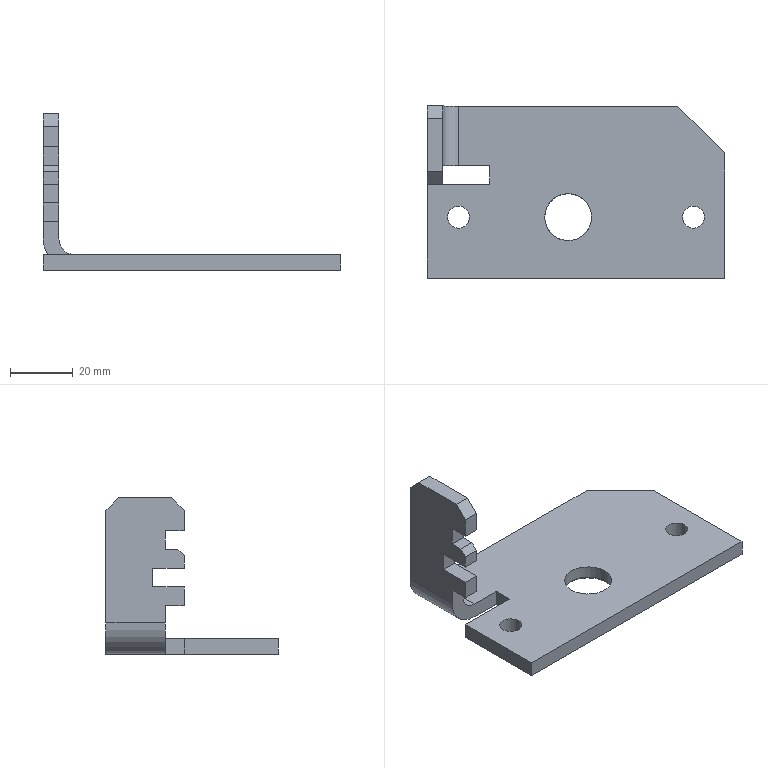Part | STEP file | 8XS100010 | 1 solid | 36 faces | box 95 x 55 x 50 mm | volume 28104 mm3 | plane 26 | cylinder 8 | cone 2 | commonest cylinder face diameters 7 x4 15 x2 10 x1 20 x1